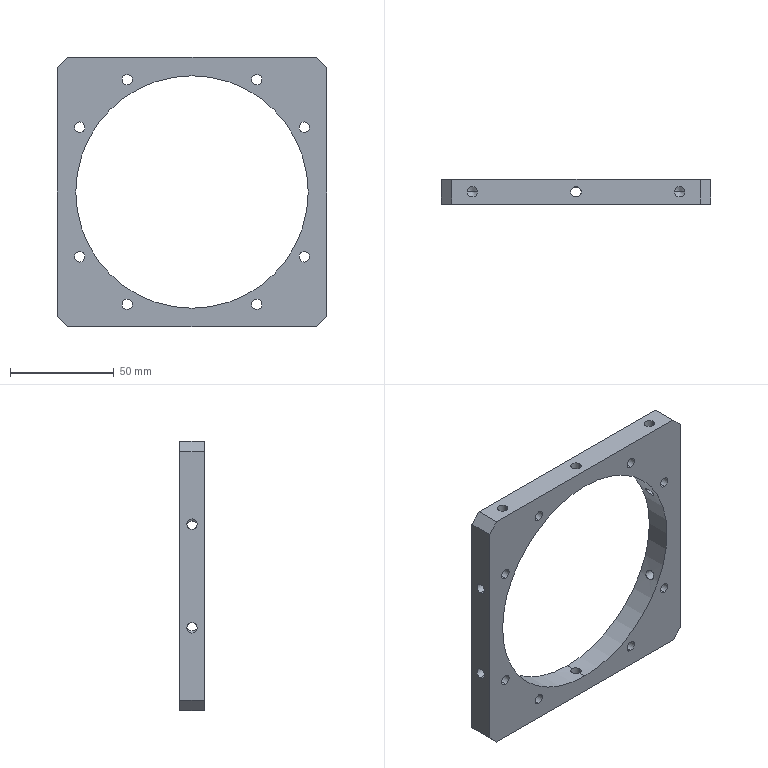Part | SolidWorks | features HoleWzd 5, Chamfer 1, Extrusion 1, ICE 1 | 1 solid | 62 faces | box 130 x 12 x 130 mm | volume 79357 mm3 | cylinder 38 | cone 14 | plane 10 | commonest cylinder face diameters 5 x36 112 x2